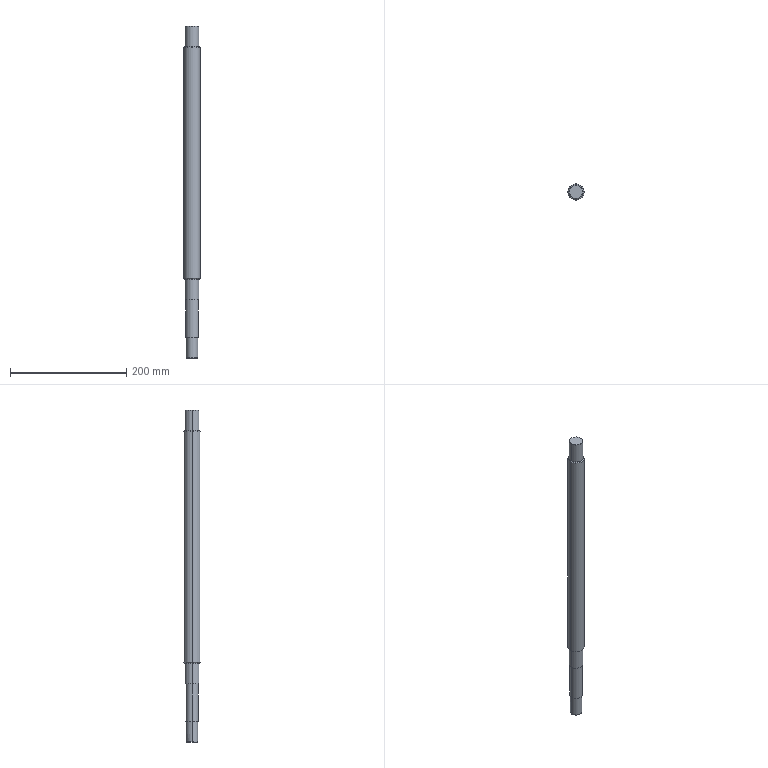Part | SolidWorks | features Chamfer 4, ICE 4, Extrusion 1 | 1 solid | 31 faces | box 28 x 28 x 572 mm | volume 313729 mm3 | cone 11 | cylinder 11 | plane 9 | commonest cylinder face diameters 24 x4 20 x2 22 x2 28 x2 6 x1
STEP:
#1=CARTESIAN_POINT('',(-9.5,0.,-572.));
#2=VERTEX_POINT('',#1);
#3=CARTESIAN_POINT('',(-3.,9.014,-572.));
#4=VERTEX_POINT('',#3);
#5=CARTESIAN_POINT('',(0.,0.,-572.));
#6=DIRECTION('',(0.,0.,-1.));
#7=DIRECTION('',(-1.,0.,0.));
#8=AXIS2_PLACEMENT_3D('',#5,#6,#7);
#9=CIRCLE('',#8,9.5);
#10=EDGE_CURVE('',#2,#4,#9,.T.);
#11=ORIENTED_EDGE('',*,*,#10,.F.);
#12=CARTESIAN_POINT('',(-10.,0.,-571.5));
#13=VERTEX_POINT('',#12);
#14=CARTESIAN_POINT('',(-9.5,0.,-572.));
#15=DIRECTION('',(-0.7071,0.,0.7071));
#16=VECTOR('',#15,1000.);
#17=LINE('',#14,#16);
#18=EDGE_CURVE('',#2,#13,#17,.T.);
#19=ORIENTED_EDGE('',*,*,#18,.T.);
#20=CARTESIAN_POINT('',(-3.,9.539,-571.5));
#21=VERTEX_POINT('',#20);
#22=CARTESIAN_POINT('',(0.,0.,-571.5));
#23=DIRECTION('',(0.,0.,1.));
#24=DIRECTION('',(-1.,0.,0.));
#25=AXIS2_PLACEMENT_3D('',#22,#23,#24);
#26=CIRCLE('',#25,10.);
#27=EDGE_CURVE('',#21,#13,#26,.T.);
#28=ORIENTED_EDGE('',*,*,#27,.F.);
#29=CARTESIAN_POINT('',(-3.,9.014,-572.));
#30=CARTESIAN_POINT('',(-3.,9.189,-571.834));
#31=CARTESIAN_POINT('',(-3.,9.364,-571.667));
#32=CARTESIAN_POINT('',(-3.,9.539,-571.5));
#33=B_SPLINE_CURVE_WITH_KNOTS('',3,(#29,#30,#31,#32),.UNSPECIFIED.,.F.,.F.,(4,4),(0.,0.0007254),.UNSPECIFIED.);
#34=EDGE_CURVE('',#4,#21,#33,.T.);
#35=ORIENTED_EDGE('',*,*,#34,.F.);
#36=EDGE_LOOP('',(#11,#19,#28,#35));
#37=FACE_OUTER_BOUND('',#36,.T.);
#38=CARTESIAN_POINT('',(0.,0.,-572.));
#39=DIRECTION('',(0.,0.,1.));
#40=DIRECTION('',(1.,0.,0.));
#41=AXIS2_PLACEMENT_3D('',#38,#39,#40);
#42=CONICAL_SURFACE('',#41,9.5,0.7854);
#43=ADVANCED_FACE('',(#37),#42,.T.);
#44=ORIENTED_EDGE('',*,*,#18,.F.);
#45=CARTESIAN_POINT('',(9.5,0.,-572.));
#46=VERTEX_POINT('',#45);
#47=CARTESIAN_POINT('',(0.,0.,-572.));
#48=DIRECTION('',(0.,0.,-1.));
#49=DIRECTION('',(-1.,0.,0.));
#50=AXIS2_PLACEMENT_3D('',#47,#48,#49);
#51=CIRCLE('',#50,9.5);
#52=EDGE_CURVE('',#46,#2,#51,.T.);
#53=ORIENTED_EDGE('',*,*,#52,.F.);
#54=CARTESIAN_POINT('',(10.,0.,-571.5));
#55=VERTEX_POINT('',#54);
#56=CARTESIAN_POINT('',(9.5,0.,-572.));
#57=DIRECTION('',(0.7071,0.,0.7071));
#58=VECTOR('',#57,1000.);
#59=LINE('',#56,#58);
#60=EDGE_CURVE('',#46,#55,#59,.T.);
#61=ORIENTED_EDGE('',*,*,#60,.T.);
#62=CARTESIAN_POINT('',(0.,0.,-571.5));
#63=DIRECTION('',(0.,0.,1.));
#64=DIRECTION('',(-1.,0.,0.));
#65=AXIS2_PLACEMENT_3D('',#62,#63,#64);
#66=CIRCLE('',#65,10.);
#67=EDGE_CURVE('',#13,#55,#66,.T.);
#68=ORIENTED_EDGE('',*,*,#67,.F.);
#69=EDGE_LOOP('',(#44,#53,#61,#68));
#70=FACE_OUTER_BOUND('',#69,.T.);
#71=CARTESIAN_POINT('',(0.,0.,-572.));
#72=DIRECTION('',(0.,0.,1.));
#73=DIRECTION('',(1.,0.,0.));
#74=AXIS2_PLACEMENT_3D('',#71,#72,#73);
#75=CONICAL_SURFACE('',#74,9.5,0.7854);
#76=ADVANCED_FACE('',(#70),#75,.T.);
#77=CARTESIAN_POINT('',(-11.5,0.,-472.));
#78=VERTEX_POINT('',#77);
#79=CARTESIAN_POINT('',(11.5,0.,-472.));
#80=VERTEX_POINT('',#79);
#81=CARTESIAN_POINT('',(0.,0.,-472.));
#82=DIRECTION('',(0.,0.,-1.));
#83=DIRECTION('',(0.,1.,0.));
#84=AXIS2_PLACEMENT_3D('',#81,#82,#83);
#85=CIRCLE('',#84,11.5);
#86=EDGE_CURVE('',#78,#80,#85,.T.);
#87=ORIENTED_EDGE('',*,*,#86,.F.);
#88=CARTESIAN_POINT('',(-12.,0.,-471.5));
#89=VERTEX_POINT('',#88);
#90=CARTESIAN_POINT('',(-12.,0.,-471.5));
#91=DIRECTION('',(-0.7071,0.,0.7071));
#92=VECTOR('',#91,1000.);
#93=LINE('',#90,#92);
#94=EDGE_CURVE('',#78,#89,#93,.T.);
#95=ORIENTED_EDGE('',*,*,#94,.T.);
#96=CARTESIAN_POINT('',(12.,0.,-471.5));
#97=VERTEX_POINT('',#96);
#98=CARTESIAN_POINT('',(0.,0.,-471.5));
#99=DIRECTION('',(0.,0.,1.));
#100=DIRECTION('',(-1.,0.,0.));
#101=AXIS2_PLACEMENT_3D('',#98,#99,#100);
#102=CIRCLE('',#101,12.);
#103=EDGE_CURVE('',#97,#89,#102,.T.);
#104=ORIENTED_EDGE('',*,*,#103,.F.);
#105=CARTESIAN_POINT('',(12.,0.,-471.5));
#106=DIRECTION('',(0.7071,0.,0.7071));
#107=VECTOR('',#106,1000.);
#108=LINE('',#105,#107);
#109=EDGE_CURVE('',#80,#97,#108,.T.);
#110=ORIENTED_EDGE('',*,*,#109,.F.);
#111=EDGE_LOOP('',(#87,#95,#104,#110));
#112=FACE_OUTER_BOUND('',#111,.T.);
#113=CARTESIAN_POINT('',(0.,0.,-471.5));
#114=DIRECTION('',(0.,0.,1.));
#115=DIRECTION('',(1.,0.,0.));
#116=AXIS2_PLACEMENT_3D('',#113,#114,#115);
#117=CONICAL_SURFACE('',#116,12.,0.7854);
#118=ADVANCED_FACE('',(#112),#117,.T.);
#119=CARTESIAN_POINT('',(11.5,0.,0.));
#120=VERTEX_POINT('',#119);
#121=CARTESIAN_POINT('',(-11.5,0.,0.));
#122=VERTEX_POINT('',#121);
#123=CARTESIAN_POINT('',(0.,0.,0.));
#124=DIRECTION('',(0.,0.,1.));
#125=DIRECTION('',(1.,0.,0.));
#126=AXIS2_PLACEMENT_3D('',#123,#124,#125);
#127=CIRCLE('',#126,11.5);
#128=EDGE_CURVE('',#120,#122,#127,.T.);
#129=ORIENTED_EDGE('',*,*,#128,.F.);
#130=CARTESIAN_POINT('',(12.,0.,-0.5));
#131=VERTEX_POINT('',#130);
#132=CARTESIAN_POINT('',(11.5,0.,0.));
#133=DIRECTION('',(0.7071,0.,-0.7071));
#134=VECTOR('',#133,1000.);
#135=LINE('',#132,#134);
#136=EDGE_CURVE('',#120,#131,#135,.T.);
#137=ORIENTED_EDGE('',*,*,#136,.T.);
#138=CARTESIAN_POINT('',(-12.,0.,-0.5));
#139=VERTEX_POINT('',#138);
#140=CARTESIAN_POINT('',(0.,0.,-0.5));
#141=DIRECTION('',(0.,0.,-1.));
#142=DIRECTION('',(1.,0.,0.));
#143=AXIS2_PLACEMENT_3D('',#140,#141,#142);
#144=CIRCLE('',#143,12.);
#145=EDGE_CURVE('',#139,#131,#144,.T.);
#146=ORIENTED_EDGE('',*,*,#145,.F.);
#147=CARTESIAN_POINT('',(-11.5,0.,0.));
#148=DIRECTION('',(-0.7071,0.,-0.7071));
#149=VECTOR('',#148,1000.);
#150=LINE('',#147,#149);
#151=EDGE_CURVE('',#122,#139,#150,.T.);
#152=ORIENTED_EDGE('',*,*,#151,.F.);
#153=EDGE_LOOP('',(#129,#137,#146,#152));
#154=FACE_OUTER_BOUND('',#153,.T.);
#155=CARTESIAN_POINT('',(0.,0.,0.));
#156=DIRECTION('',(0.,0.,-1.));
#157=DIRECTION('',(-1.,0.,0.));
#158=AXIS2_PLACEMENT_3D('',#155,#156,#157);
#159=CONICAL_SURFACE('',#158,11.5,0.7854);
#160=ADVANCED_FACE('',(#154),#159,.T.);
#161=CARTESIAN_POINT('',(13.,0.,-36.));
#162=VERTEX_POINT('',#161);
#163=CARTESIAN_POINT('',(-13.,0.,-36.));
#164=VERTEX_POINT('',#163);
#165=CARTESIAN_POINT('',(0.,0.,-36.));
#166=DIRECTION('',(0.,0.,1.));
#167=DIRECTION('',(1.,0.,0.));
#168=AXIS2_PLACEMENT_3D('',#165,#166,#167);
#169=CIRCLE('',#168,13.);
#170=EDGE_CURVE('',#162,#164,#169,.T.);
#171=ORIENTED_EDGE('',*,*,#170,.F.);
#172=CARTESIAN_POINT('',(14.,0.,-37.));
#173=VERTEX_POINT('',#172);
#174=CARTESIAN_POINT('',(13.,0.,-36.));
#175=DIRECTION('',(0.7071,0.,-0.7071));
#176=VECTOR('',#175,1000.);
#177=LINE('',#174,#176);
#178=EDGE_CURVE('',#162,#173,#177,.T.);
#179=ORIENTED_EDGE('',*,*,#178,.T.);
#180=CARTESIAN_POINT('',(-14.,0.,-37.));
#181=VERTEX_POINT('',#180);
#182=CARTESIAN_POINT('',(0.,0.,-37.));
#183=DIRECTION('',(0.,0.,-1.));
#184=DIRECTION('',(1.,0.,0.));
#185=AXIS2_PLACEMENT_3D('',#182,#183,#184);
#186=CIRCLE('',#185,14.);
#187=EDGE_CURVE('',#181,#173,#186,.T.);
#188=ORIENTED_EDGE('',*,*,#187,.F.);
#189=CARTESIAN_POINT('',(-13.,0.,-36.));
#190=DIRECTION('',(-0.7071,0.,-0.7071));
#191=VECTOR('',#190,1000.);
#192=LINE('',#189,#191);
#193=EDGE_CURVE('',#164,#181,#192,.T.);
#194=ORIENTED_EDGE('',*,*,#193,.F.);
#195=EDGE_LOOP('',(#171,#179,#188,#194));
#196=FACE_OUTER_BOUND('',#195,.T.);
#197=CARTESIAN_POINT('',(0.,0.,-36.));
#198=DIRECTION('',(0.,0.,-1.));
#199=DIRECTION('',(-1.,0.,0.));
#200=AXIS2_PLACEMENT_3D('',#197,#198,#199);
#201=CONICAL_SURFACE('',#200,13.,0.7854);
#202=ADVANCED_FACE('',(#196),#201,.T.);
#203=CARTESIAN_POINT('',(-13.,0.,-436.));
#204=VERTEX_POINT('',#203);
#205=CARTESIAN_POINT('',(13.,0.,-436.));
#206=VERTEX_POINT('',#205);
#207=CARTESIAN_POINT('',(0.,0.,-436.));
#208=DIRECTION('',(0.,0.,-1.));
#209=DIRECTION('',(1.,0.,0.));
#210=AXIS2_PLACEMENT_3D('',#207,#208,#209);
#211=CIRCLE('',#210,13.);
#212=EDGE_CURVE('',#204,#206,#211,.T.);
#213=ORIENTED_EDGE('',*,*,#212,.F.);
#214=CARTESIAN_POINT('',(-14.,0.,-435.));
#215=VERTEX_POINT('',#214);
#216=CARTESIAN_POINT('',(-14.,0.,-435.));
#217=DIRECTION('',(-0.7071,0.,0.7071));
#218=VECTOR('',#217,1000.);
#219=LINE('',#216,#218);
#220=EDGE_CURVE('',#204,#215,#219,.T.);
#221=ORIENTED_EDGE('',*,*,#220,.T.);
#222=CARTESIAN_POINT('',(14.,0.,-435.));
#223=VERTEX_POINT('',#222);
#224=CARTESIAN_POINT('',(0.,0.,-435.));
#225=DIRECTION('',(0.,0.,1.));
#226=DIRECTION('',(1.,0.,0.));
#227=AXIS2_PLACEMENT_3D('',#224,#225,#226);
#228=CIRCLE('',#227,14.);
#229=EDGE_CURVE('',#223,#215,#228,.T.);
#230=ORIENTED_EDGE('',*,*,#229,.F.);
#231=CARTESIAN_POINT('',(14.,0.,-435.));
#232=DIRECTION('',(0.7071,0.,0.7071));
#233=VECTOR('',#232,1000.);
#234=LINE('',#231,#233);
#235=EDGE_CURVE('',#206,#223,#234,.T.);
#236=ORIENTED_EDGE('',*,*,#235,.F.);
#237=EDGE_LOOP('',(#213,#221,#230,#236));
#238=FACE_OUTER_BOUND('',#237,.T.);
#239=CARTESIAN_POINT('',(0.,0.,-435.));
#240=DIRECTION('',(0.,0.,1.));
#241=DIRECTION('',(1.,0.,0.));
#242=AXIS2_PLACEMENT_3D('',#239,#240,#241);
#243=CONICAL_SURFACE('',#242,14.,0.7854);
#244=ADVANCED_FACE('',(#238),#243,.T.);
#245=CARTESIAN_POINT('',(-12.,0.,-36.));
#246=VERTEX_POINT('',#245);
#247=CARTESIAN_POINT('',(12.,0.,-36.));
#248=VERTEX_POINT('',#247);
#249=CARTESIAN_POINT('',(0.,0.,-36.));
#250=DIRECTION('',(0.,0.,-1.));
#251=DIRECTION('',(1.,0.,0.));
#252=AXIS2_PLACEMENT_3D('',#249,#250,#251);
#253=CIRCLE('',#252,12.);
#254=EDGE_CURVE('',#246,#248,#253,.T.);
#255=ORIENTED_EDGE('',*,*,#254,.F.);
#256=CARTESIAN_POINT('',(-12.,0.,-505.941));
#257=DIRECTION('',(0.,0.,1.));
#258=VECTOR('',#257,1000.);
#259=LINE('',#256,#258);
#260=EDGE_CURVE('',#246,#139,#259,.T.);
#261=ORIENTED_EDGE('',*,*,#260,.T.);
#262=ORIENTED_EDGE('',*,*,#145,.T.);
#263=CARTESIAN_POINT('',(12.,0.,-505.941));
#264=DIRECTION('',(0.,0.,1.));
#265=VECTOR('',#264,1000.);
#266=LINE('',#263,#265);
#267=EDGE_CURVE('',#248,#131,#266,.T.);
#268=ORIENTED_EDGE('',*,*,#267,.F.);
#269=EDGE_LOOP('',(#255,#261,#262,#268));
#270=FACE_OUTER_BOUND('',#269,.T.);
#271=CARTESIAN_POINT('',(0.,0.,-505.941));
#272=DIRECTION('',(0.,0.,1.));
#273=DIRECTION('',(1.,0.,0.));
#274=AXIS2_PLACEMENT_3D('',#271,#272,#273);
#275=CYLINDRICAL_SURFACE('',#274,12.);
#276=ADVANCED_FACE('',(#270),#275,.T.);
#277=ORIENTED_EDGE('',*,*,#229,.T.);
#278=CARTESIAN_POINT('',(-14.,0.,-436.));
#279=DIRECTION('',(0.,0.,1.));
#280=VECTOR('',#279,1000.);
#281=LINE('',#278,#280);
#282=EDGE_CURVE('',#215,#181,#281,.T.);
#283=ORIENTED_EDGE('',*,*,#282,.T.);
#284=ORIENTED_EDGE('',*,*,#187,.T.);
#285=CARTESIAN_POINT('',(14.,0.,-436.));
#286=DIRECTION('',(0.,0.,1.));
#287=VECTOR('',#286,1000.);
#288=LINE('',#285,#287);
#289=EDGE_CURVE('',#223,#173,#288,.T.);
#290=ORIENTED_EDGE('',*,*,#289,.F.);
#291=EDGE_LOOP('',(#277,#283,#284,#290));
#292=FACE_OUTER_BOUND('',#291,.T.);
#293=CARTESIAN_POINT('',(0.,0.,-436.));
#294=DIRECTION('',(0.,0.,1.));
#295=DIRECTION('',(1.,0.,0.));
#296=AXIS2_PLACEMENT_3D('',#293,#294,#295);
#297=CYLINDRICAL_SURFACE('',#296,14.);
#298=ADVANCED_FACE('',(#292),#297,.T.);
#299=ORIENTED_EDGE('',*,*,#103,.T.);
#300=CARTESIAN_POINT('',(-12.,0.,-436.));
#301=VERTEX_POINT('',#300);
#302=CARTESIAN_POINT('',(-12.,0.,-505.941));
#303=DIRECTION('',(0.,0.,1.));
#304=VECTOR('',#303,1000.);
#305=LINE('',#302,#304);
#306=EDGE_CURVE('',#89,#301,#305,.T.);
#307=ORIENTED_EDGE('',*,*,#306,.T.);
#308=CARTESIAN_POINT('',(12.,0.,-436.));
#309=VERTEX_POINT('',#308);
#310=CARTESIAN_POINT('',(0.,0.,-436.));
#311=DIRECTION('',(0.,0.,-1.));
#312=DIRECTION('',(1.,0.,0.));
#313=AXIS2_PLACEMENT_3D('',#310,#311,#312);
#314=CIRCLE('',#313,12.);
#315=EDGE_CURVE('',#301,#309,#314,.T.);
#316=ORIENTED_EDGE('',*,*,#315,.T.);
#317=CARTESIAN_POINT('',(12.,0.,-505.941));
#318=DIRECTION('',(0.,0.,1.));
#319=VECTOR('',#318,1000.);
#320=LINE('',#317,#319);
#321=EDGE_CURVE('',#97,#309,#320,.T.);
#322=ORIENTED_EDGE('',*,*,#321,.F.);
#323=EDGE_LOOP('',(#299,#307,#316,#322));
#324=FACE_OUTER_BOUND('',#323,.T.);
#325=CARTESIAN_POINT('',(0.,0.,-505.941));
#326=DIRECTION('',(0.,0.,1.));
#327=DIRECTION('',(1.,0.,0.));
#328=AXIS2_PLACEMENT_3D('',#325,#326,#327);
#329=CYLINDRICAL_SURFACE('',#328,12.);
#330=ADVANCED_FACE('',(#324),#329,.T.);
#331=CARTESIAN_POINT('',(-11.,0.,-536.));
#332=VERTEX_POINT('',#331);
#333=CARTESIAN_POINT('',(11.,0.,-536.));
#334=VERTEX_POINT('',#333);
#335=CARTESIAN_POINT('',(0.,0.,-536.));
#336=DIRECTION('',(0.,0.,-1.));
#337=DIRECTION('',(-1.,0.,0.));
#338=AXIS2_PLACEMENT_3D('',#335,#336,#337);
#339=CIRCLE('',#338,11.);
#340=EDGE_CURVE('',#332,#334,#339,.T.);
#341=ORIENTED_EDGE('',*,*,#340,.F.);
#342=CARTESIAN_POINT('',(-11.,0.,-472.));
#343=VERTEX_POINT('',#342);
#344=CARTESIAN_POINT('',(-11.,0.,-572.));
#345=DIRECTION('',(0.,0.,1.));
#346=VECTOR('',#345,1000.);
#347=LINE('',#344,#346);
#348=EDGE_CURVE('',#332,#343,#347,.T.);
#349=ORIENTED_EDGE('',*,*,#348,.T.);
#350=CARTESIAN_POINT('',(11.,0.,-472.));
#351=VERTEX_POINT('',#350);
#352=CARTESIAN_POINT('',(0.,0.,-472.));
#353=DIRECTION('',(0.,0.,-1.));
#354=DIRECTION('',(-1.,0.,0.));
#355=AXIS2_PLACEMENT_3D('',#352,#353,#354);
#356=CIRCLE('',#355,11.);
#357=EDGE_CURVE('',#343,#351,#356,.T.);
#358=ORIENTED_EDGE('',*,*,#357,.T.);
#359=CARTESIAN_POINT('',(11.,0.,-572.));
#360=DIRECTION('',(0.,0.,1.));
#361=VECTOR('',#360,1000.);
#362=LINE('',#359,#361);
#363=EDGE_CURVE('',#334,#351,#362,.T.);
#364=ORIENTED_EDGE('',*,*,#363,.F.);
#365=EDGE_LOOP('',(#341,#349,#358,#364));
#366=FACE_OUTER_BOUND('',#365,.T.);
#367=CARTESIAN_POINT('',(0.,0.,-572.));
#368=DIRECTION('',(0.,0.,1.));
#369=DIRECTION('',(1.,0.,0.));
#370=AXIS2_PLACEMENT_3D('',#367,#368,#369);
#371=CYLINDRICAL_SURFACE('',#370,11.);
#372=ADVANCED_FACE('',(#366),#371,.T.);
#373=CARTESIAN_POINT('',(-10.,0.,-536.));
#374=VERTEX_POINT('',#373);
#375=CARTESIAN_POINT('',(10.,0.,-536.));
#376=VERTEX_POINT('',#375);
#377=CARTESIAN_POINT('',(0.,0.,-536.));
#378=DIRECTION('',(0.,0.,-1.));
#379=DIRECTION('',(-1.,0.,0.));
#380=AXIS2_PLACEMENT_3D('',#377,#378,#379);
#381=CIRCLE('',#380,10.);
#382=EDGE_CURVE('',#374,#376,#381,.T.);
#383=ORIENTED_EDGE('',*,*,#382,.T.);
#384=CARTESIAN_POINT('',(10.,0.,-536.));
#385=DIRECTION('',(0.,0.,-1.));
#386=VECTOR('',#385,1000.);
#387=LINE('',#384,#386);
#388=EDGE_CURVE('',#376,#55,#387,.T.);
#389=ORIENTED_EDGE('',*,*,#388,.T.);
#390=CARTESIAN_POINT('',(3.,9.539,-571.5));
#391=VERTEX_POINT('',#390);
#392=CARTESIAN_POINT('',(0.,0.,-571.5));
#393=DIRECTION('',(0.,0.,1.));
#394=DIRECTION('',(-1.,0.,0.));
#395=AXIS2_PLACEMENT_3D('',#392,#393,#394);
#396=CIRCLE('',#395,10.);
#397=EDGE_CURVE('',#55,#391,#396,.T.);
#398=ORIENTED_EDGE('',*,*,#397,.T.);
#399=CARTESIAN_POINT('',(3.,9.539,-541.));
#400=VERTEX_POINT('',#399);
#401=CARTESIAN_POINT('',(3.,9.539,-536.));
#402=DIRECTION('',(0.,0.,1.));
#403=VECTOR('',#402,1000.);
#404=LINE('',#401,#403);
#405=EDGE_CURVE('',#391,#400,#404,.T.);
#406=ORIENTED_EDGE('',*,*,#405,.T.);
#407=CARTESIAN_POINT('',(-3.,9.539,-541.));
#408=VERTEX_POINT('',#407);
#409=CARTESIAN_POINT('',(3.,9.539,-541.));
#410=CARTESIAN_POINT('',(3.,9.539,-540.801));
#411=CARTESIAN_POINT('',(2.98,9.546,-540.605));
#412=CARTESIAN_POINT('',(2.903,9.569,-540.22));
#413=CARTESIAN_POINT('',(2.845,9.587,-540.029));
#414=CARTESIAN_POINT('',(2.694,9.631,-539.666));
#415=CARTESIAN_POINT('',(2.602,9.656,-539.494));
#416=CARTESIAN_POINT('',(2.385,9.712,-539.169));
#417=CARTESIAN_POINT('',(2.259,9.743,-539.016));
#418=CARTESIAN_POINT('',(1.847,9.832,-538.604));
#419=CARTESIAN_POINT('',(1.514,9.891,-538.381));
#420=CARTESIAN_POINT('',(0.9732,9.954,-538.156));
#421=CARTESIAN_POINT('',(0.783,9.971,-538.097));
#422=CARTESIAN_POINT('',(0.3953,9.994,-538.02));
#423=CARTESIAN_POINT('',(0.1999,10.,-538.));
#424=CARTESIAN_POINT('',(-0.194,10.,-538.));
#425=CARTESIAN_POINT('',(-0.394,9.994,-538.019));
#426=CARTESIAN_POINT('',(-0.7797,9.971,-538.096));
#427=CARTESIAN_POINT('',(-0.9673,9.955,-538.153));
#428=CARTESIAN_POINT('',(-1.332,9.913,-538.305));
#429=CARTESIAN_POINT('',(-1.506,9.887,-538.398));
#430=CARTESIAN_POINT('',(-1.83,9.833,-538.614));
#431=CARTESIAN_POINT('',(-1.982,9.803,-538.74));
#432=CARTESIAN_POINT('',(-2.259,9.743,-539.016));
#433=CARTESIAN_POINT('',(-2.383,9.713,-539.167));
#434=CARTESIAN_POINT('',(-2.6,9.657,-539.49));
#435=CARTESIAN_POINT('',(-2.694,9.631,-539.666));
#436=CARTESIAN_POINT('',(-2.845,9.587,-540.027));
#437=CARTESIAN_POINT('',(-2.902,9.57,-540.214));
#438=CARTESIAN_POINT('',(-2.98,9.546,-540.601));
#439=CARTESIAN_POINT('',(-3.,9.539,-540.801));
#440=CARTESIAN_POINT('',(-3.,9.539,-541.));
#441=B_SPLINE_CURVE_WITH_KNOTS('',3,(#409,#410,#411,#412,#413,#414,#415,#416,#417,#418,#419,#420,#421,#422,#423,#424,#425,#426,#427,#428,#429,#430,#431,#432,#433,#434,#435,#436,#437,#438,#439,#440),.UNSPECIFIED.,.F.,.F.,(4,2,2,2,2,2,2,2,2,2,2,2,2,2,2,4),(0.,0.0005894,0.001179,0.001768,0.002358,0.003536,0.004126,0.004715,0.005305,0.005894,0.006484,0.007073,0.007662,0.008252,0.008841,0.009431),.UNSPECIFIED.);
#442=EDGE_CURVE('',#400,#408,#441,.T.);
#443=ORIENTED_EDGE('',*,*,#442,.T.);
#444=CARTESIAN_POINT('',(-3.,9.539,-536.));
#445=DIRECTION('',(0.,0.,-1.));
#446=VECTOR('',#445,1000.);
#447=LINE('',#444,#446);
#448=EDGE_CURVE('',#408,#21,#447,.T.);
#449=ORIENTED_EDGE('',*,*,#448,.T.);
#450=ORIENTED_EDGE('',*,*,#27,.T.);
#451=CARTESIAN_POINT('',(-10.,0.,-536.));
#452=DIRECTION('',(0.,0.,-1.));
#453=VECTOR('',#452,1000.);
#454=LINE('',#451,#453);
#455=EDGE_CURVE('',#374,#13,#454,.T.);
#456=ORIENTED_EDGE('',*,*,#455,.F.);
#457=EDGE_LOOP('',(#383,#389,#398,#406,#443,#449,#450,#456));
#458=FACE_OUTER_BOUND('',#457,.T.);
#459=CARTESIAN_POINT('',(0.,0.,-536.));
#460=DIRECTION('',(0.,0.,-1.));
#461=DIRECTION('',(-1.,0.,0.));
#462=AXIS2_PLACEMENT_3D('',#459,#460,#461);
#463=CYLINDRICAL_SURFACE('',#462,10.);
#464=ADVANCED_FACE('',(#458),#463,.T.);
#465=ORIENTED_EDGE('',*,*,#388,.F.);
#466=CARTESIAN_POINT('',(0.,0.,-536.));
#467=DIRECTION('',(0.,0.,-1.));
#468=DIRECTION('',(-1.,0.,0.));
#469=AXIS2_PLACEMENT_3D('',#466,#467,#468);
#470=CIRCLE('',#469,10.);
#471=EDGE_CURVE('',#376,#374,#470,.T.);
#472=ORIENTED_EDGE('',*,*,#471,.T.);
#473=ORIENTED_EDGE('',*,*,#455,.T.);
#474=ORIENTED_EDGE('',*,*,#67,.T.);
#475=EDGE_LOOP('',(#465,#472,#473,#474));
#476=FACE_OUTER_BOUND('',#475,.T.);
#477=CARTESIAN_POINT('',(0.,0.,-536.));
#478=DIRECTION('',(0.,0.,-1.));
#479=DIRECTION('',(-1.,0.,0.));
#480=AXIS2_PLACEMENT_3D('',#477,#478,#479);
#481=CYLINDRICAL_SURFACE('',#480,10.);
#482=ADVANCED_FACE('',(#476),#481,.T.);
#483=CARTESIAN_POINT('',(3.,6.5,-572.));
#484=VERTEX_POINT('',#483);
#485=CARTESIAN_POINT('',(3.,9.014,-572.));
#486=VERTEX_POINT('',#485);
#487=CARTESIAN_POINT('',(3.,0.,-572.));
#488=DIRECTION('',(0.,1.,0.));
#489=VECTOR('',#488,1000.);
#490=LINE('',#487,#489);
#491=EDGE_CURVE('',#484,#486,#490,.T.);
#492=ORIENTED_EDGE('',*,*,#491,.T.);
#493=CARTESIAN_POINT('',(0.,0.,-572.));
#494=DIRECTION('',(0.,0.,-1.));
#495=DIRECTION('',(-1.,0.,0.));
#496=AXIS2_PLACEMENT_3D('',#493,#494,#495);
#497=CIRCLE('',#496,9.5);
#498=EDGE_CURVE('',#486,#46,#497,.T.);
#499=ORIENTED_EDGE('',*,*,#498,.T.);
#500=ORIENTED_EDGE('',*,*,#52,.T.);
#501=ORIENTED_EDGE('',*,*,#10,.T.);
#502=CARTESIAN_POINT('',(-3.,6.5,-572.));
#503=VERTEX_POINT('',#502);
#504=CARTESIAN_POINT('',(-3.,0.,-572.));
#505=DIRECTION('',(0.,-1.,0.));
#506=VECTOR('',#505,1000.);
#507=LINE('',#504,#506);
#508=EDGE_CURVE('',#4,#503,#507,.T.);
#509=ORIENTED_EDGE('',*,*,#508,.T.);
#510=CARTESIAN_POINT('',(0.,6.5,-572.));
#511=DIRECTION('',(1.,0.,0.));
#512=VECTOR('',#511,1000.);
#513=LINE('',#510,#512);
#514=EDGE_CURVE('',#503,#484,#513,.T.);
#515=ORIENTED_EDGE('',*,*,#514,.T.);
#516=EDGE_LOOP('',(#492,#499,#500,#501,#509,#515));
#517=FACE_OUTER_BOUND('',#516,.T.);
#518=CARTESIAN_POINT('',(0.,0.,-572.));
#519=DIRECTION('',(0.,0.,-1.));
#520=DIRECTION('',(-1.,0.,0.));
#521=AXIS2_PLACEMENT_3D('',#518,#519,#520);
#522=PLANE('',#521);
#523=ADVANCED_FACE('',(#517),#522,.T.);
#524=ORIENTED_EDGE('',*,*,#348,.F.);
#525=CARTESIAN_POINT('',(0.,0.,-536.));
#526=DIRECTION('',(0.,0.,-1.));
#527=DIRECTION('',(-1.,0.,0.));
#528=AXIS2_PLACEMENT_3D('',#525,#526,#527);
#529=CIRCLE('',#528,11.);
#530=EDGE_CURVE('',#334,#332,#529,.T.);
#531=ORIENTED_EDGE('',*,*,#530,.F.);
#532=ORIENTED_EDGE('',*,*,#363,.T.);
#533=CARTESIAN_POINT('',(0.,0.,-472.));
#534=DIRECTION('',(0.,0.,-1.));
#535=DIRECTION('',(-1.,0.,0.));
#536=AXIS2_PLACEMENT_3D('',#533,#534,#535);
#537=CIRCLE('',#536,11.);
#538=EDGE_CURVE('',#351,#343,#537,.T.);
#539=ORIENTED_EDGE('',*,*,#538,.T.);
#540=EDGE_LOOP('',(#524,#531,#532,#539));
#541=FACE_OUTER_BOUND('',#540,.T.);
#542=CARTESIAN_POINT('',(0.,0.,-572.));
#543=DIRECTION('',(0.,0.,1.));
#544=DIRECTION('',(1.,0.,0.));
#545=AXIS2_PLACEMENT_3D('',#542,#543,#544);
#546=CYLINDRICAL_SURFACE('',#545,11.);
#547=ADVANCED_FACE('',(#541),#546,.T.);
#548=ORIENTED_EDGE('',*,*,#306,.F.);
#549=CARTESIAN_POINT('',(0.,0.,-471.5));
#550=DIRECTION('',(0.,0.,1.));
#551=DIRECTION('',(-1.,0.,0.));
#552=AXIS2_PLACEMENT_3D('',#549,#550,#551);
#553=CIRCLE('',#552,12.);
#554=EDGE_CURVE('',#89,#97,#553,.T.);
#555=ORIENTED_EDGE('',*,*,#554,.T.);
#556=ORIENTED_EDGE('',*,*,#321,.T.);
#557=CARTESIAN_POINT('',(0.,0.,-436.));
#558=DIRECTION('',(0.,0.,-1.));
#559=DIRECTION('',(1.,0.,0.));
#560=AXIS2_PLACEMENT_3D('',#557,#558,#559);
#561=CIRCLE('',#560,12.);
#562=EDGE_CURVE('',#309,#301,#561,.T.);
#563=ORIENTED_EDGE('',*,*,#562,.T.);
#564=EDGE_LOOP('',(#548,#555,#556,#563));
#565=FACE_OUTER_BOUND('',#564,.T.);
#566=CARTESIAN_POINT('',(0.,0.,-505.941));
#567=DIRECTION('',(0.,0.,1.));
#568=DIRECTION('',(1.,0.,0.));
#569=AXIS2_PLACEMENT_3D('',#566,#567,#568);
#570=CYLINDRICAL_SURFACE('',#569,12.);
#571=ADVANCED_FACE('',(#565),#570,.T.);
#572=CARTESIAN_POINT('',(0.,0.,-472.));
#573=DIRECTION('',(0.,0.,-1.));
#574=DIRECTION('',(0.,1.,0.));
#575=AXIS2_PLACEMENT_3D('',#572,#573,#574);
#576=CIRCLE('',#575,11.5);
#577=EDGE_CURVE('',#80,#78,#576,.T.);
#578=ORIENTED_EDGE('',*,*,#577,.T.);
#579=ORIENTED_EDGE('',*,*,#86,.T.);
#580=EDGE_LOOP('',(#578,#579));
#581=FACE_OUTER_BOUND('',#580,.T.);
#582=ORIENTED_EDGE('',*,*,#538,.F.);
#583=ORIENTED_EDGE('',*,*,#357,.F.);
#584=EDGE_LOOP('',(#582,#583));
#585=FACE_BOUND('',#584,.T.);
#586=CARTESIAN_POINT('',(10.217,6.294,-472.));
#587=DIRECTION('',(0.,0.,-1.));
#588=DIRECTION('',(-0.5245,0.8514,0.));
#589=AXIS2_PLACEMENT_3D('',#586,#587,#588);
#590=PLANE('',#589);
#591=ADVANCED_FACE('',(#581,#585),#590,.T.);
#592=ORIENTED_EDGE('',*,*,#282,.F.);
#593=CARTESIAN_POINT('',(0.,0.,-435.));
#594=DIRECTION('',(0.,0.,1.));
#595=DIRECTION('',(1.,0.,0.));
#596=AXIS2_PLACEMENT_3D('',#593,#594,#595);
#597=CIRCLE('',#596,14.);
#598=EDGE_CURVE('',#215,#223,#597,.T.);
#599=ORIENTED_EDGE('',*,*,#598,.T.);
#600=ORIENTED_EDGE('',*,*,#289,.T.);
#601=CARTESIAN_POINT('',(0.,0.,-37.));
#602=DIRECTION('',(0.,0.,-1.));
#603=DIRECTION('',(1.,0.,0.));
#604=AXIS2_PLACEMENT_3D('',#601,#602,#603);
#605=CIRCLE('',#604,14.);
#606=EDGE_CURVE('',#173,#181,#605,.T.);
#607=ORIENTED_EDGE('',*,*,#606,.T.);
#608=EDGE_LOOP('',(#592,#599,#600,#607));
#609=FACE_OUTER_BOUND('',#608,.T.);
#610=CARTESIAN_POINT('',(0.,0.,-436.));
#611=DIRECTION('',(0.,0.,1.));
#612=DIRECTION('',(1.,0.,0.));
#613=AXIS2_PLACEMENT_3D('',#610,#611,#612);
#614=CYLINDRICAL_SURFACE('',#613,14.);
#615=ADVANCED_FACE('',(#609),#614,.T.);
#616=CARTESIAN_POINT('',(0.,0.,-436.));
#617=DIRECTION('',(0.,0.,-1.));
#618=DIRECTION('',(1.,0.,0.));
#619=AXIS2_PLACEMENT_3D('',#616,#617,#618);
#620=CIRCLE('',#619,13.);
#621=EDGE_CURVE('',#206,#204,#620,.T.);
#622=ORIENTED_EDGE('',*,*,#621,.T.);
#623=ORIENTED_EDGE('',*,*,#212,.T.);
#624=EDGE_LOOP('',(#622,#623));
#625=FACE_OUTER_BOUND('',#624,.T.);
#626=ORIENTED_EDGE('',*,*,#562,.F.);
#627=ORIENTED_EDGE('',*,*,#315,.F.);
#628=EDGE_LOOP('',(#626,#627));
#629=FACE_BOUND('',#628,.T.);
#630=CARTESIAN_POINT('',(0.,0.,-436.));
#631=DIRECTION('',(0.,0.,1.));
#632=DIRECTION('',(1.,0.,0.));
#633=AXIS2_PLACEMENT_3D('',#630,#631,#632);
#634=PLANE('',#633);
#635=ADVANCED_FACE('',(#625,#629),#634,.F.);
#636=CARTESIAN_POINT('',(0.,0.,-36.));
#637=DIRECTION('',(0.,0.,1.));
#638=DIRECTION('',(1.,0.,0.));
#639=AXIS2_PLACEMENT_3D('',#636,#637,#638);
#640=CIRCLE('',#639,13.);
#641=EDGE_CURVE('',#164,#162,#640,.T.);
#642=ORIENTED_EDGE('',*,*,#641,.T.);
#643=ORIENTED_EDGE('',*,*,#170,.T.);
#644=EDGE_LOOP('',(#642,#643));
#645=FACE_OUTER_BOUND('',#644,.T.);
#646=CARTESIAN_POINT('',(0.,0.,-36.));
#647=DIRECTION('',(0.,0.,-1.));
#648=DIRECTION('',(1.,0.,0.));
#649=AXIS2_PLACEMENT_3D('',#646,#647,#648);
#650=CIRCLE('',#649,12.);
#651=EDGE_CURVE('',#248,#246,#650,.T.);
#652=ORIENTED_EDGE('',*,*,#651,.T.);
#653=ORIENTED_EDGE('',*,*,#254,.T.);
#654=EDGE_LOOP('',(#652,#653));
#655=FACE_BOUND('',#654,.T.);
#656=CARTESIAN_POINT('',(0.,0.,-36.));
#657=DIRECTION('',(0.,0.,1.));
#658=DIRECTION('',(1.,0.,0.));
#659=AXIS2_PLACEMENT_3D('',#656,#657,#658);
#660=PLANE('',#659);
#661=ADVANCED_FACE('',(#645,#655),#660,.T.);
#662=CARTESIAN_POINT('',(0.,0.,0.));
#663=DIRECTION('',(0.,0.,1.));
#664=DIRECTION('',(1.,0.,0.));
#665=AXIS2_PLACEMENT_3D('',#662,#663,#664);
#666=CIRCLE('',#665,11.5);
#667=EDGE_CURVE('',#122,#120,#666,.T.);
#668=ORIENTED_EDGE('',*,*,#667,.T.);
#669=ORIENTED_EDGE('',*,*,#128,.T.);
#670=EDGE_LOOP('',(#668,#669));
#671=FACE_OUTER_BOUND('',#670,.T.);
#672=CARTESIAN_POINT('',(0.,0.,0.));
#673=DIRECTION('',(0.,0.,1.));
#674=DIRECTION('',(1.,0.,0.));
#675=AXIS2_PLACEMENT_3D('',#672,#673,#674);
#676=PLANE('',#675);
#677=ADVANCED_FACE('',(#671),#676,.T.);
#678=ORIENTED_EDGE('',*,*,#260,.F.);
#679=ORIENTED_EDGE('',*,*,#651,.F.);
#680=ORIENTED_EDGE('',*,*,#267,.T.);
#681=CARTESIAN_POINT('',(0.,0.,-0.5));
#682=DIRECTION('',(0.,0.,-1.));
#683=DIRECTION('',(1.,0.,0.));
#684=AXIS2_PLACEMENT_3D('',#681,#682,#683);
#685=CIRCLE('',#684,12.);
#686=EDGE_CURVE('',#131,#139,#685,.T.);
#687=ORIENTED_EDGE('',*,*,#686,.T.);
#688=EDGE_LOOP('',(#678,#679,#680,#687));
#689=FACE_OUTER_BOUND('',#688,.T.);
#690=CARTESIAN_POINT('',(0.,0.,-505.941));
#691=DIRECTION('',(0.,0.,1.));
#692=DIRECTION('',(1.,0.,0.));
#693=AXIS2_PLACEMENT_3D('',#690,#691,#692);
#694=CYLINDRICAL_SURFACE('',#693,12.);
#695=ADVANCED_FACE('',(#689),#694,.T.);
#696=ORIENTED_EDGE('',*,*,#220,.F.);
#697=ORIENTED_EDGE('',*,*,#621,.F.);
#698=ORIENTED_EDGE('',*,*,#235,.T.);
#699=ORIENTED_EDGE('',*,*,#598,.F.);
#700=EDGE_LOOP('',(#696,#697,#698,#699));
#701=FACE_OUTER_BOUND('',#700,.T.);
#702=CARTESIAN_POINT('',(0.,0.,-435.));
#703=DIRECTION('',(0.,0.,1.));
#704=DIRECTION('',(1.,0.,0.));
#705=AXIS2_PLACEMENT_3D('',#702,#703,#704);
#706=CONICAL_SURFACE('',#705,14.,0.7854);
#707=ADVANCED_FACE('',(#701),#706,.T.);
#708=ORIENTED_EDGE('',*,*,#178,.F.);
#709=ORIENTED_EDGE('',*,*,#641,.F.);
#710=ORIENTED_EDGE('',*,*,#193,.T.);
#711=ORIENTED_EDGE('',*,*,#606,.F.);
#712=EDGE_LOOP('',(#708,#709,#710,#711));
#713=FACE_OUTER_BOUND('',#712,.T.);
#714=CARTESIAN_POINT('',(0.,0.,-36.));
#715=DIRECTION('',(0.,0.,-1.));
#716=DIRECTION('',(-1.,0.,0.));
#717=AXIS2_PLACEMENT_3D('',#714,#715,#716);
#718=CONICAL_SURFACE('',#717,13.,0.7854);
#719=ADVANCED_FACE('',(#713),#718,.T.);
#720=ORIENTED_EDGE('',*,*,#136,.F.);
#721=ORIENTED_EDGE('',*,*,#667,.F.);
#722=ORIENTED_EDGE('',*,*,#151,.T.);
#723=ORIENTED_EDGE('',*,*,#686,.F.);
#724=EDGE_LOOP('',(#720,#721,#722,#723));
#725=FACE_OUTER_BOUND('',#724,.T.);
#726=CARTESIAN_POINT('',(0.,0.,0.));
#727=DIRECTION('',(0.,0.,-1.));
#728=DIRECTION('',(-1.,0.,0.));
#729=AXIS2_PLACEMENT_3D('',#726,#727,#728);
#730=CONICAL_SURFACE('',#729,11.5,0.7854);
#731=ADVANCED_FACE('',(#725),#730,.T.);
#732=ORIENTED_EDGE('',*,*,#94,.F.);
#733=ORIENTED_EDGE('',*,*,#577,.F.);
#734=ORIENTED_EDGE('',*,*,#109,.T.);
#735=ORIENTED_EDGE('',*,*,#554,.F.);
#736=EDGE_LOOP('',(#732,#733,#734,#735));
#737=FACE_OUTER_BOUND('',#736,.T.);
#738=CARTESIAN_POINT('',(0.,0.,-471.5));
#739=DIRECTION('',(0.,0.,1.));
#740=DIRECTION('',(1.,0.,0.));
#741=AXIS2_PLACEMENT_3D('',#738,#739,#740);
#742=CONICAL_SURFACE('',#741,12.,0.7854);
#743=ADVANCED_FACE('',(#737),#742,.T.);
#744=ORIENTED_EDGE('',*,*,#382,.F.);
#745=ORIENTED_EDGE('',*,*,#471,.F.);
#746=EDGE_LOOP('',(#744,#745));
#747=FACE_BOUND('',#746,.T.);
#748=ORIENTED_EDGE('',*,*,#530,.T.);
#749=ORIENTED_EDGE('',*,*,#340,.T.);
#750=EDGE_LOOP('',(#748,#749));
#751=FACE_OUTER_BOUND('',#750,.T.);
#752=CARTESIAN_POINT('',(0.,0.,-536.));
#753=DIRECTION('',(0.,0.,-1.));
#754=DIRECTION('',(-1.,0.,0.));
#755=AXIS2_PLACEMENT_3D('',#752,#753,#754);
#756=PLANE('',#755);
#757=ADVANCED_FACE('',(#747,#751),#756,.T.);
#758=ORIENTED_EDGE('',*,*,#508,.F.);
#759=ORIENTED_EDGE('',*,*,#34,.T.);
#760=ORIENTED_EDGE('',*,*,#448,.F.);
#761=CARTESIAN_POINT('',(-3.,6.5,-541.));
#762=VERTEX_POINT('',#761);
#763=CARTESIAN_POINT('',(-3.,14.,-541.));
#764=DIRECTION('',(0.,-1.,0.));
#765=VECTOR('',#764,1000.);
#766=LINE('',#763,#765);
#767=EDGE_CURVE('',#408,#762,#766,.T.);
#768=ORIENTED_EDGE('',*,*,#767,.T.);
#769=CARTESIAN_POINT('',(-3.,6.5,-576.648));
#770=DIRECTION('',(0.,0.,1.));
#771=VECTOR('',#770,1000.);
#772=LINE('',#769,#771);
#773=EDGE_CURVE('',#503,#762,#772,.T.);
#774=ORIENTED_EDGE('',*,*,#773,.F.);
#775=EDGE_LOOP('',(#758,#759,#760,#768,#774));
#776=FACE_OUTER_BOUND('',#775,.T.);
#777=CARTESIAN_POINT('',(-3.,14.,-576.648));
#778=DIRECTION('',(1.,0.,0.));
#779=DIRECTION('',(0.,0.,-1.));
#780=AXIS2_PLACEMENT_3D('',#777,#778,#779);
#781=PLANE('',#780);
#782=ADVANCED_FACE('',(#776),#781,.T.);
#783=CARTESIAN_POINT('',(3.,6.5,-541.));
#784=VERTEX_POINT('',#783);
#785=CARTESIAN_POINT('',(3.,14.,-541.));
#786=DIRECTION('',(0.,-1.,0.));
#787=VECTOR('',#786,1000.);
#788=LINE('',#785,#787);
#789=EDGE_CURVE('',#400,#784,#788,.T.);
#790=ORIENTED_EDGE('',*,*,#789,.T.);
#791=CARTESIAN_POINT('',(0.,6.5,-541.));
#792=DIRECTION('',(0.,1.,0.));
#793=DIRECTION('',(0.,0.,1.));
#794=AXIS2_PLACEMENT_3D('',#791,#792,#793);
#795=CIRCLE('',#794,3.);
#796=EDGE_CURVE('',#762,#784,#795,.T.);
#797=ORIENTED_EDGE('',*,*,#796,.F.);
#798=ORIENTED_EDGE('',*,*,#767,.F.);
#799=ORIENTED_EDGE('',*,*,#442,.F.);
#800=EDGE_LOOP('',(#790,#797,#798,#799));
#801=FACE_OUTER_BOUND('',#800,.T.);
#802=CARTESIAN_POINT('',(0.,14.,-541.));
#803=DIRECTION('',(0.,-1.,0.));
#804=DIRECTION('',(0.,0.,-1.));
#805=AXIS2_PLACEMENT_3D('',#802,#803,#804);
#806=CYLINDRICAL_SURFACE('',#805,3.);
#807=ADVANCED_FACE('',(#801),#806,.F.);
#808=ORIENTED_EDGE('',*,*,#405,.F.);
#809=CARTESIAN_POINT('',(3.,9.539,-571.5));
#810=CARTESIAN_POINT('',(3.,9.364,-571.667));
#811=CARTESIAN_POINT('',(3.,9.189,-571.834));
#812=CARTESIAN_POINT('',(3.,9.014,-572.));
#813=B_SPLINE_CURVE_WITH_KNOTS('',3,(#809,#810,#811,#812),.UNSPECIFIED.,.F.,.F.,(4,4),(0.,0.0007254),.UNSPECIFIED.);
#814=EDGE_CURVE('',#391,#486,#813,.T.);
#815=ORIENTED_EDGE('',*,*,#814,.T.);
#816=ORIENTED_EDGE('',*,*,#491,.F.);
#817=CARTESIAN_POINT('',(3.,6.5,-576.648));
#818=DIRECTION('',(0.,0.,-1.));
#819=VECTOR('',#818,1000.);
#820=LINE('',#817,#819);
#821=EDGE_CURVE('',#784,#484,#820,.T.);
#822=ORIENTED_EDGE('',*,*,#821,.F.);
#823=ORIENTED_EDGE('',*,*,#789,.F.);
#824=EDGE_LOOP('',(#808,#815,#816,#822,#823));
#825=FACE_OUTER_BOUND('',#824,.T.);
#826=CARTESIAN_POINT('',(3.,14.,-576.648));
#827=DIRECTION('',(-1.,0.,0.));
#828=DIRECTION('',(0.,0.,1.));
#829=AXIS2_PLACEMENT_3D('',#826,#827,#828);
#830=PLANE('',#829);
#831=ADVANCED_FACE('',(#825),#830,.T.);
#832=ORIENTED_EDGE('',*,*,#773,.T.);
#833=ORIENTED_EDGE('',*,*,#796,.T.);
#834=ORIENTED_EDGE('',*,*,#821,.T.);
#835=ORIENTED_EDGE('',*,*,#514,.F.);
#836=EDGE_LOOP('',(#832,#833,#834,#835));
#837=FACE_OUTER_BOUND('',#836,.T.);
#838=CARTESIAN_POINT('',(0.,6.5,-576.648));
#839=DIRECTION('',(0.,1.,0.));
#840=DIRECTION('',(0.,0.,1.));
#841=AXIS2_PLACEMENT_3D('',#838,#839,#840);
#842=PLANE('',#841);
#843=ADVANCED_FACE('',(#837),#842,.T.);
#844=ORIENTED_EDGE('',*,*,#60,.F.);
#845=ORIENTED_EDGE('',*,*,#498,.F.);
#846=ORIENTED_EDGE('',*,*,#814,.F.);
#847=ORIENTED_EDGE('',*,*,#397,.F.);
#848=EDGE_LOOP('',(#844,#845,#846,#847));
#849=FACE_OUTER_BOUND('',#848,.T.);
#850=CARTESIAN_POINT('',(0.,0.,-572.));
#851=DIRECTION('',(0.,0.,1.));
#852=DIRECTION('',(1.,0.,0.));
#853=AXIS2_PLACEMENT_3D('',#850,#851,#852);
#854=CONICAL_SURFACE('',#853,9.5,0.7854);
#855=ADVANCED_FACE('',(#849),#854,.T.);
#856=CLOSED_SHELL('',(#43,#76,#118,#160,#202,#244,#276,#298,#330,#372,#464,#482,#523,#547,#571,#591,#615,#635,#661,#677,#695,#707,#719,#731,#743,#757,#782,#807,#831,#843,#855));
#857=MANIFOLD_SOLID_BREP('',#856);
#858=CARTESIAN_POINT('',(0.,0.,0.));
#859=DIRECTION('',(0.,0.,1.));
#860=DIRECTION('',(1.,0.,0.));
#861=AXIS2_PLACEMENT_3D('',#858,#859,#860);
#862=(LENGTH_UNIT()NAMED_UNIT(*)SI_UNIT(.MILLI.,.METRE.));
#863=UNCERTAINTY_MEASURE_WITH_UNIT(LENGTH_MEASURE(0.00001),#862,'','');
#864=(NAMED_UNIT(*)PLANE_ANGLE_UNIT()SI_UNIT($,.RADIAN.));
#865=(NAMED_UNIT(*)SI_UNIT($,.STERADIAN.)SOLID_ANGLE_UNIT());
#866=(GEOMETRIC_REPRESENTATION_CONTEXT(3)GLOBAL_UNCERTAINTY_ASSIGNED_CONTEXT((#863))GLOBAL_UNIT_ASSIGNED_CONTEXT((#862,#864,#865))REPRESENTATION_CONTEXT('',''));
#867=ADVANCED_BREP_SHAPE_REPRESENTATION('',(#857,#861),#866);